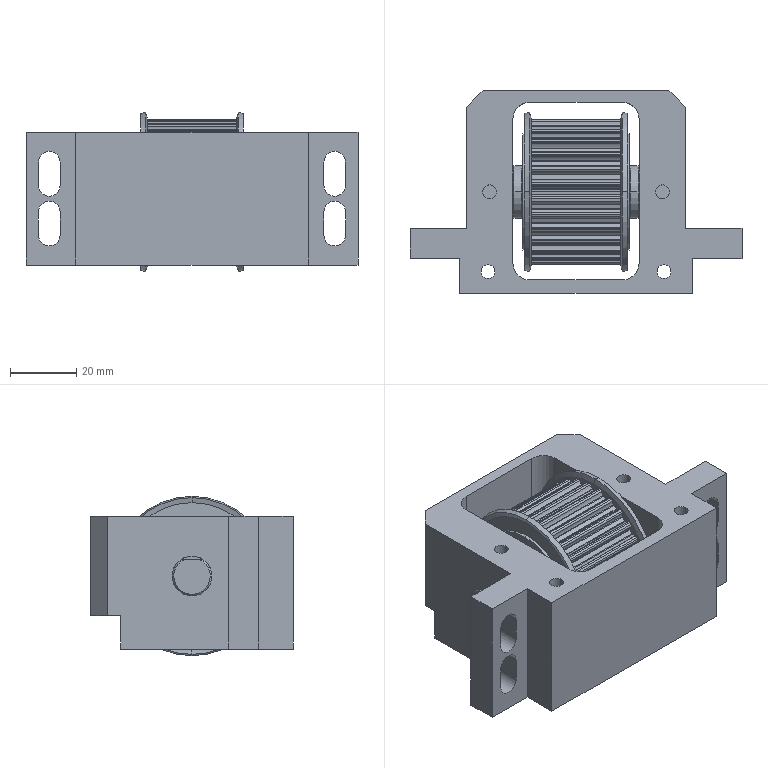Part | SolidWorks | 7 solids | 542 faces | box 100 x 61 x 48 mm | volume 123898 mm3 | cylinder 333 | cone 82 | plane 67 | torus 60 | commonest cylinder face diameters 1.1 x68 0.5 x64 6.55 x60 40.06 x29 43.6 x28 12 x10